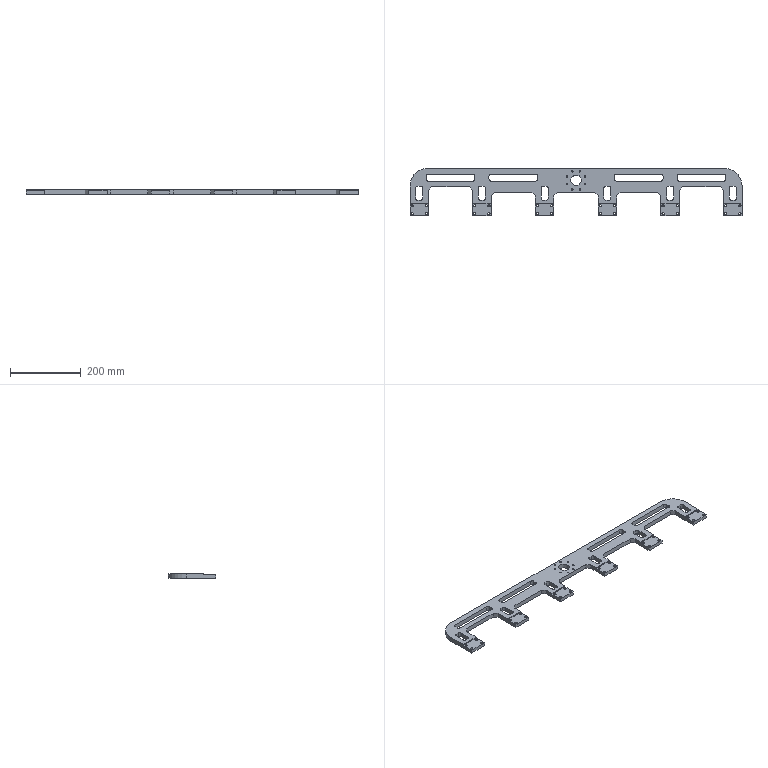NC program | NX | posted with a generic post | part box 941 x 134 x 13 mm
Lines 73 to 1151 of 4152:
(ZLEVEL_PROFILE_COPY_3_COPY_1 , TOOL : D10)
N132 T10 M6
N134 G54
N136 G17 G0 G90 X50.491 Y75.6 S9500 M3
N138 G43 Z30. H10
N140 Z4.036
N142 G94 G1 Z-0.964 F1000.
N144 X52.223 Y72.6
N146 G3 X53.089 Y72.1 R1.
N148 G1 X420.5 F3500.
N150 G2 X475.6 Y17. R55.1
N152 G1 Y-67.
N154 G2 X470.5 Y-72.1 R5.1
N156 G1 X418.5
N158 G2 X413.4 Y-67. R5.1
N160 G1 Y2.888
N162 X406.387 Y9.9
N164 X304.813
N166 X297.8 Y2.888
N168 Y-67.
N170 G2 X292.7 Y-72.1 R5.1
N172 G1 X240.7
N174 G2 X235.6 Y-67. R5.1
N176 G1 Y-13.067
N178 X228.588 Y-6.055
N180 X127.013
N182 X120. Y-13.068
N184 Y-67.
N186 G2 X114.9 Y-72.1 R5.1
N188 G1 X62.9
N190 G2 X57.8 Y-67. R5.1
N192 G1 Y-13.067
N194 X53.089 Y-8.357
N196 G3 X52.123 Y-8.098 R1.
N198 G1 X46.687 Y-9.555
N200 Z4.036
N202 G0 Z30.
N204 Z3.071
N206 G1 Z-1.929 F1000.
N208 X52.123 Y-8.098
N210 G2 X53.089 Y-8.357 R1.
N212 G1 X57.8 Y-13.067 F3500.
N214 Y-67.
N216 G3 X62.9 Y-72.1 R5.1
N218 G1 X114.9
N220 G3 X120. Y-67. R5.1
N222 G1 Y-13.068
N224 X127.013 Y-6.055
N226 X228.588
N228 X235.6 Y-13.067
N230 Y-67.
N232 G3 X240.7 Y-72.1 R5.1
N234 G1 X292.7
N236 G3 X297.8 Y-67. R5.1
N238 G1 Y2.888
N240 X304.813 Y9.9
N242 X406.387
N244 X413.4 Y2.888
N246 Y-67.
N248 G3 X418.5 Y-72.1 R5.1
N250 G1 X470.5
N252 G3 X475.6 Y-67. R5.1
N254 G1 Y17.
N256 G3 X420.5 Y72.1 R55.1
N258 G1 X53.089
N260 G2 X52.223 Y72.6 R1.
N262 G1 X50.491 Y75.6
N264 Z3.071
N266 G0 Z30.
N268 Z2.107
N270 G1 Z-2.893 F1000.
N272 X52.223 Y72.6
N274 G3 X53.089 Y72.1 R1.
N276 G1 X420.5 F3500.
N278 G2 X475.6 Y17. R55.1
N280 G1 Y-67.
N282 G2 X470.5 Y-72.1 R5.1
N284 G1 X418.5
N286 G2 X413.4 Y-67. R5.1
N288 G1 Y2.888
N290 X406.387 Y9.9
N292 X304.813
N294 X297.8 Y2.888
N296 Y-67.
N298 G2 X292.7 Y-72.1 R5.1
N300 G1 X240.7
N302 G2 X235.6 Y-67. R5.1
N304 G1 Y-13.067
N306 X228.588 Y-6.055
N308 X127.013
N310 X120. Y-13.068
N312 Y-67.
N314 G2 X114.9 Y-72.1 R5.1
N316 G1 X62.9
N318 G2 X57.8 Y-67. R5.1
N320 G1 Y-13.067
N322 X53.089 Y-8.357
N324 G3 X52.123 Y-8.098 R1.
N326 G1 X46.687 Y-9.555
N328 Z2.107
N330 G0 Z30.
N332 Z1.143
N334 G1 Z-3.857 F1000.
N336 X52.123 Y-8.098
N338 G2 X53.089 Y-8.357 R1.
N340 G1 X57.8 Y-13.067 F3500.
N342 Y-67.
N344 G3 X62.9 Y-72.1 R5.1
N346 G1 X114.9
N348 G3 X120. Y-67. R5.1
N350 G1 Y-13.068
N352 X127.013 Y-6.055
N354 X228.588
N356 X235.6 Y-13.067
N358 Y-67.
N360 G3 X240.7 Y-72.1 R5.1
N362 G1 X292.7
N364 G3 X297.8 Y-67. R5.1
N366 G1 Y2.888
N368 X304.813 Y9.9
N370 X406.387
N372 X413.4 Y2.888
N374 Y-67.
N376 G3 X418.5 Y-72.1 R5.1
N378 G1 X470.5
N380 G3 X475.6 Y-67. R5.1
N382 G1 Y17.
N384 G3 X420.5 Y72.1 R55.1
N386 G1 X53.089
N388 G2 X52.223 Y72.6 R1.
N390 G1 X50.491 Y75.6
N392 Z1.143
N394 G0 Z30.
N396 Z0.179
N398 G1 Z-4.821 F1000.
N400 X52.223 Y72.6
N402 G3 X53.089 Y72.1 R1.
N404 G1 X420.5 F3500.
N406 G2 X475.6 Y17. R55.1
N408 G1 Y-67.
N410 G2 X470.5 Y-72.1 R5.1
N412 G1 X418.5
N414 G2 X413.4 Y-67. R5.1
N416 G1 Y2.888
N418 X406.387 Y9.9
N420 X304.813
N422 X297.8 Y2.888
N424 Y-67.
N426 G2 X292.7 Y-72.1 R5.1
N428 G1 X240.7
N430 G2 X235.6 Y-67. R5.1
N432 G1 Y-13.067
N434 X228.588 Y-6.055
N436 X127.013
N438 X120. Y-13.068
N440 Y-67.
N442 G2 X114.9 Y-72.1 R5.1
N444 G1 X62.9
N446 G2 X57.8 Y-67. R5.1
N448 G1 Y-13.067
N450 X53.089 Y-8.357
N452 G3 X52.123 Y-8.098 R1.
N454 G1 X46.687 Y-9.555
N456 Z0.179
N458 G0 Z30.
N460 Z-0.786
N462 G1 Z-5.786 F1000.
N464 X52.123 Y-8.098
N466 G2 X53.089 Y-8.357 R1.
N468 G1 X57.8 Y-13.067 F3500.
N470 Y-67.
N472 G3 X62.9 Y-72.1 R5.1
N474 G1 X114.9
N476 G3 X120. Y-67. R5.1
N478 G1 Y-13.068
N480 X127.013 Y-6.055
N482 X228.588
N484 X235.6 Y-13.067
N486 Y-67.
N488 G3 X240.7 Y-72.1 R5.1
N490 G1 X292.7
N492 G3 X297.8 Y-67. R5.1
N494 G1 Y2.888
N496 X304.813 Y9.9
N498 X406.387
N500 X413.4 Y2.888
N502 Y-67.
N504 G3 X418.5 Y-72.1 R5.1
N506 G1 X470.5
N508 G3 X475.6 Y-67. R5.1
N510 G1 Y17.
N512 G3 X420.5 Y72.1 R55.1
N514 G1 X53.089
N516 G2 X52.223 Y72.6 R1.
N518 G1 X50.491 Y75.6
N520 Z-0.786
N522 G0 Z30.
N524 Z-1.75
N526 G1 Z-6.75 F1000.
N528 X52.223 Y72.6
N530 G3 X53.089 Y72.1 R1.
N532 G1 X420.5 F3500.
N534 G2 X475.6 Y17. R55.1
N536 G1 Y-67.
N538 G2 X470.5 Y-72.1 R5.1
N540 G1 X418.5
N542 G2 X413.4 Y-67. R5.1
N544 G1 Y2.888
N546 X406.387 Y9.9
N548 X304.813
N550 X297.8 Y2.888
N552 Y-67.
N554 G2 X292.7 Y-72.1 R5.1
N556 G1 X240.7
N558 G2 X235.6 Y-67. R5.1
N560 G1 Y-13.067
N562 X228.588 Y-6.055
N564 X127.013
N566 X120. Y-13.068
N568 Y-67.
N570 G2 X114.9 Y-72.1 R5.1
N572 G1 X62.9
N574 G2 X57.8 Y-67. R5.1
N576 G1 Y-13.067
N578 X53.089 Y-8.357
N580 G3 X52.123 Y-8.098 R1.
N582 G1 X46.687 Y-9.555
N584 Z-1.75
N586 G0 Z30.
N588 Z-2.714
N590 G1 Z-7.714 F1000.
N592 X52.123 Y-8.098
N594 G2 X53.089 Y-8.357 R1.
N596 G1 X57.8 Y-13.067 F3500.
N598 Y-67.
N600 G3 X62.9 Y-72.1 R5.1
N602 G1 X114.9
N604 G3 X120. Y-67. R5.1
N606 G1 Y-13.068
N608 X127.013 Y-6.055
N610 X228.588
N612 X235.6 Y-13.067
N614 Y-67.
N616 G3 X240.7 Y-72.1 R5.1
N618 G1 X292.7
N620 G3 X297.8 Y-67. R5.1
N622 G1 Y2.888
N624 X304.813 Y9.9
N626 X406.387
N628 X413.4 Y2.888
N630 Y-67.
N632 G3 X418.5 Y-72.1 R5.1
N634 G1 X470.5
N636 G3 X475.6 Y-67. R5.1
N638 G1 Y17.
N640 G3 X420.5 Y72.1 R55.1
N642 G1 X53.089
N644 G2 X52.223 Y72.6 R1.
N646 G1 X50.491 Y75.6
N648 Z-2.714
N650 G0 Z30.
N652 Z-3.679
N654 G1 Z-8.679 F1000.
N656 X52.223 Y72.6
N658 G3 X53.089 Y72.1 R1.
N660 G1 X420.5 F3500.
N662 G2 X475.6 Y17. R55.1
N664 G1 Y-67.
N666 G2 X470.5 Y-72.1 R5.1
N668 G1 X418.5
N670 G2 X413.4 Y-67. R5.1
N672 G1 Y2.888
N674 X406.388 Y9.9
N676 X304.812
N678 X297.8 Y2.888
N680 Y-67.
N682 G2 X292.7 Y-72.1 R5.1
N684 G1 X240.7
N686 G2 X235.6 Y-67. R5.1
N688 G1 Y-13.067
N690 X228.588 Y-6.055
N692 X127.012
N694 X120. Y-13.067
N696 Y-67.
N698 G2 X114.9 Y-72.1 R5.1
N700 G1 X62.9
N702 G2 X57.8 Y-67. R5.1
N704 G1 Y-13.067
N706 X53.089 Y-8.357
N708 G3 X52.123 Y-8.098 R1.
N710 G1 X46.686 Y-9.555
N712 Z-3.679
N714 G0 Z30.
N716 Z-4.643
N718 G1 Z-9.643 F1000.
N720 X52.123 Y-8.098
N722 G2 X53.089 Y-8.357 R1.
N724 G1 X57.8 Y-13.067 F3500.
N726 Y-67.
N728 G3 X62.9 Y-72.1 R5.1
N730 G1 X114.9
N732 G3 X120. Y-67. R5.1
N734 G1 Y-13.067
N736 X127.012 Y-6.055
N738 X228.588
N740 X235.6 Y-13.067
N742 Y-67.
N744 G3 X240.7 Y-72.1 R5.1
N746 G1 X292.7
N748 G3 X297.8 Y-67. R5.1
N750 G1 Y2.888
N752 X304.812 Y9.9
N754 X406.388
N756 X413.4 Y2.888
N758 Y-67.
N760 G3 X418.5 Y-72.1 R5.1
N762 G1 X470.5
N764 G3 X475.6 Y-67. R5.1
N766 G1 Y17.
N768 G3 X420.5 Y72.1 R55.1
N770 G1 X53.089
N772 G2 X52.223 Y72.6 R1.
N774 G1 X50.491 Y75.6
N776 Z-4.643
N778 G0 Z30.
N780 Z-5.607
N782 G1 Z-10.607 F1000.
N784 X52.223 Y72.6
N786 G3 X53.089 Y72.1 R1.
N788 G1 X420.5 F3500.
N790 G2 X475.6 Y17. R55.1
N792 G1 Y-67.
N794 G2 X470.5 Y-72.1 R5.1
N796 G1 X418.5
N798 G2 X413.4 Y-67. R5.1
N800 G1 Y2.888
N802 X406.388 Y9.9
N804 X304.812
N806 X297.8 Y2.888
N808 Y-67.
N810 G2 X292.7 Y-72.1 R5.1
N812 G1 X240.7
N814 G2 X235.6 Y-67. R5.1
N816 G1 Y-13.067
N818 X228.588 Y-6.055
N820 X127.012
N822 X120. Y-13.067
N824 Y-67.
N826 G2 X114.9 Y-72.1 R5.1
N828 G1 X62.9
N830 G2 X57.8 Y-67. R5.1
N832 G1 Y-13.067
N834 X53.089 Y-8.357
N836 G3 X52.123 Y-8.098 R1.
N838 G1 X46.686 Y-9.555
N840 Z-5.607
N842 G0 Z30.
N844 Z-6.571
N846 G1 Z-11.571 F1000.
N848 X52.123 Y-8.098
N850 G2 X53.089 Y-8.357 R1.
N852 G1 X57.8 Y-13.067 F3500.
N854 Y-67.
N856 G3 X62.9 Y-72.1 R5.1
N858 G1 X114.9
N860 G3 X120. Y-67. R5.1
N862 G1 Y-13.067
N864 X127.012 Y-6.055
N866 X228.588
N868 X235.6 Y-13.067
N870 Y-67.
N872 G3 X240.7 Y-72.1 R5.1
N874 G1 X292.7
N876 G3 X297.8 Y-67. R5.1
N878 G1 Y2.888
N880 X304.812 Y9.9
N882 X406.388
N884 X413.4 Y2.888
N886 Y-67.
N888 G3 X418.5 Y-72.1 R5.1
N890 G1 X470.5
N892 G3 X475.6 Y-67. R5.1
N894 G1 Y17.
N896 G3 X420.5 Y72.1 R55.1
N898 G1 X53.089
N900 G2 X52.223 Y72.6 R1.
N902 G1 X50.491 Y75.6
N904 Z-6.571
N906 G0 Z30.
N908 Z-7.536
N910 G1 Z-12.536 F1000.
N912 X52.223 Y72.6
N914 G3 X53.089 Y72.1 R1.
N916 G1 X420.5 F3500.
N918 G2 X475.6 Y17. R55.1
N920 G1 Y-67.
N922 G2 X470.5 Y-72.1 R5.1
N924 G1 X418.5
N926 G2 X413.4 Y-67. R5.1
N928 G1 Y2.888
N930 X406.388 Y9.9
N932 X304.812
N934 X297.8 Y2.888
N936 Y-67.
N938 G2 X292.7 Y-72.1 R5.1
N940 G1 X240.7
N942 G2 X235.6 Y-67. R5.1
N944 G1 Y-13.067
N946 X228.588 Y-6.055
N948 X127.012
N950 X120. Y-13.067
N952 Y-67.
N954 G2 X114.9 Y-72.1 R5.1
N956 G1 X62.9
N958 G2 X57.8 Y-67. R5.1
N960 G1 Y-13.067
N962 X53.089 Y-8.357
N964 G3 X52.123 Y-8.098 R1.
N966 G1 X46.686 Y-9.555
N968 Z-7.536
N970 G0 Z30.
N972 Z-8.5
N974 G1 Z-13.5 F1000.
N976 X52.123 Y-8.098
N978 G2 X53.089 Y-8.357 R1.
N980 G1 X57.8 Y-13.067 F3500.
N982 Y-67.
N984 G3 X62.9 Y-72.1 R5.1
N986 G1 X114.9
N988 G3 X120. Y-67. R5.1
N990 G1 Y-13.067
N992 X127.012 Y-6.055
N994 X228.588
N996 X235.6 Y-13.067
N998 Y-67.
N1000 G3 X240.7 Y-72.1 R5.1
N1002 G1 X292.7
N1004 G3 X297.8 Y-67. R5.1
N1006 G1 Y2.888
N1008 X304.812 Y9.9
N1010 X406.388
N1012 X413.4 Y2.888
N1014 Y-67.
N1016 G3 X418.5 Y-72.1 R5.1
N1018 G1 X470.5
N1020 G3 X475.6 Y-67. R5.1
N1022 G1 Y17.
N1024 G3 X420.5 Y72.1 R55.1
N1026 G1 X53.089
N1028 G2 X52.223 Y72.6 R1.
N1030 G1 X50.491 Y75.6
N1032 Z-8.5
N1034 G0 Z30.
(ZLEVEL_PROFILE_COPY_3_COPY_COPY , TOOL : D10)
N1036 Y75.5
N1038 Z-8.5
N1040 G1 Z-13.5 F1000.
N1042 X52.223 Y72.5
N1044 G3 X53.089 Y72. R1.
N1046 G1 X420.5 F1200.
N1048 G2 X475.5 Y17. R55.
N1050 G1 Y-67.
N1052 G2 X470.5 Y-72. R5.
N1054 G1 X418.5
N1056 G2 X413.5 Y-67. R5.
N1058 G1 Y2.929
N1060 X406.429 Y10.
N1062 X304.771
N1064 X297.7 Y2.929
N1066 Y-67.
N1068 G2 X292.7 Y-72. R5.
N1070 G1 X240.7
N1072 G2 X235.7 Y-67. R5.
N1074 G1 Y-13.026
N1076 X228.629 Y-5.955
N1078 X126.971
N1080 X119.9 Y-13.026
N1082 Y-67.
N1084 G2 X114.9 Y-72. R5.
N1086 G1 X62.9
N1088 G2 X57.9 Y-67. R5.
N1090 G1 Y-13.026
N1092 X53.089 Y-8.215
N1094 G3 X52.123 Y-7.957 R1.
N1096 G1 X46.531 Y-9.455
N1098 Z-8.5
N1100 G0 Z30.
(ZLEVEL_PROFILE_COPY_2_COPY_COPY_1 , TOOL : D10)
N1102 X402.621 Y45.9
N1104 Z1.5
N1106 G1 X355.6 Z-0.964 F1000.
N1108 X292.7 F3500.
N1110 G3 X291.8 Y45. R0.9
N1112 G1 Y37.
N1114 G3 X292.7 Y36.1 R0.9
N1116 G1 X418.5
N1118 G3 X419.4 Y37. R0.9
N1120 G1 Y45.
N1122 G3 X418.5 Y45.9 R0.9
N1124 G1 X355.6
N1126 X300.356 Z-1.929
N1128 X292.7
N1130 G3 X291.8 Y45. R0.9
N1132 G1 Y37.
N1134 G3 X292.7 Y36.1 R0.9
N1136 G1 X418.5
N1138 G3 X419.4 Y37. R0.9
N1140 G1 Y45.
N1142 G3 X418.5 Y45.9 R0.9
N1144 G1 X355.6
N1146 X300.356 Z-2.893
N1148 X292.7
N1150 G3 X291.8 Y45. R0.9
N1152 G1 Y37.
N1154 G3 X292.7 Y36.1 R0.9
N1156 G1 X418.5
N1158 G3 X419.4 Y37. R0.9
N1160 G1 Y45.
N1162 G3 X418.5 Y45.9 R0.9
N1164 G1 X355.6
N1166 X300.356 Z-3.857
N1168 X292.7
N1170 G3 X291.8 Y45. R0.9
N1172 G1 Y37.
N1174 G3 X292.7 Y36.1 R0.9
N1176 G1 X418.5
N1178 G3 X419.4 Y37. R0.9
N1180 G1 Y45.
N1182 G3 X418.5 Y45.9 R0.9
N1184 G1 X355.6
N1186 X300.356 Z-4.821
N1188 X292.7
N1190 G3 X291.8 Y45. R0.9
N1192 G1 Y37.
N1194 G3 X292.7 Y36.1 R0.9
N1196 G1 X418.5
N1198 G3 X419.4 Y37. R0.9
N1200 G1 Y45.
N1202 G3 X418.5 Y45.9 R0.9
N1204 G1 X355.6
N1206 X300.356 Z-5.786
N1208 X292.7
N1210 G3 X291.8 Y45. R0.9
N1212 G1 Y37.
N1214 G3 X292.7 Y36.1 R0.9
N1216 G1 X418.5
N1218 G3 X419.4 Y37. R0.9
N1220 G1 Y45.
N1222 G3 X418.5 Y45.9 R0.9
N1224 G1 X355.6
N1226 X300.356 Z-6.75
N1228 X292.7
N1230 G3 X291.8 Y45. R0.9
N1232 G1 Y37.
N1234 G3 X292.7 Y36.1 R0.9
N1236 G1 X418.5
N1238 G3 X419.4 Y37. R0.9
N1240 G1 Y45.
N1242 G3 X418.5 Y45.9 R0.9
N1244 G1 X355.6
N1246 X300.356 Z-7.714
N1248 X292.7
N1250 G3 X291.8 Y45. R0.9
N1252 G1 Y37.
N1254 G3 X292.7 Y36.1 R0.9
N1256 G1 X418.5
N1258 G3 X419.4 Y37. R0.9
N1260 G1 Y45.
N1262 G3 X418.5 Y45.9 R0.9
N1264 G1 X355.6
N1266 X300.356 Z-8.679
N1268 X292.7
N1270 G3 X291.8 Y45. R0.9
N1272 G1 Y37.
N1274 G3 X292.7 Y36.1 R0.9
N1276 G1 X418.5
N1278 G3 X419.4 Y37. R0.9
N1280 G1 Y45.
N1282 G3 X418.5 Y45.9 R0.9
N1284 G1 X355.6
N1286 X300.356 Z-9.643
N1288 X292.7
N1290 G3 X291.8 Y45. R0.9
N1292 G1 Y37.
N1294 G3 X292.7 Y36.1 R0.9
N1296 G1 X418.5
N1298 G3 X419.4 Y37. R0.9
N1300 G1 Y45.
N1302 G3 X418.5 Y45.9 R0.9
N1304 G1 X355.6
N1306 X300.356 Z-10.607
N1308 X292.7
N1310 G3 X291.8 Y45. R0.9
N1312 G1 Y37.
N1314 G3 X292.7 Y36.1 R0.9
N1316 G1 X418.5
N1318 G3 X419.4 Y37. R0.9
N1320 G1 Y45.
N1322 G3 X418.5 Y45.9 R0.9
N1324 G1 X355.6
N1326 X300.356 Z-11.571
N1328 X292.7
N1330 G3 X291.8 Y45. R0.9
N1332 G1 Y37.
N1334 G3 X292.7 Y36.1 R0.9
N1336 G1 X418.5
N1338 G3 X419.4 Y37. R0.9
N1340 G1 Y45.
N1342 G3 X418.5 Y45.9 R0.9
N1344 G1 X355.6
N1346 X300.356 Z-12.536
N1348 X292.7
N1350 G3 X291.8 Y45. R0.9
N1352 G1 Y37.
N1354 G3 X292.7 Y36.1 R0.9
N1356 G1 X418.5
N1358 G3 X419.4 Y37. R0.9
N1360 G1 Y45.
N1362 G3 X418.5 Y45.9 R0.9
N1364 G1 X355.6
N1366 X300.356 Z-13.5
N1368 X292.7
N1370 G3 X291.8 Y45. R0.9
N1372 G1 Y37.
N1374 G3 X292.7 Y36.1 R0.9
N1376 G1 X418.5
N1378 G3 X419.4 Y37. R0.9
N1380 G1 Y45.
N1382 G3 X418.5 Y45.9 R0.9
N1384 G1 X300.356
N1386 Z-12.
N1388 G0 Z30.
N1390 X224.821
N1392 Z1.5
N1394 G1 X177.8 Z-0.964 F1000.
N1396 X114.9 F3500.
N1398 G3 X114. Y45. R0.9
N1400 G1 Y37.
N1402 G3 X114.9 Y36.1 R0.9
N1404 G1 X240.7
N1406 G3 X241.6 Y37. R0.9
N1408 G1 Y45.
N1410 G3 X240.7 Y45.9 R0.9
N1412 G1 X177.8
N1414 X122.556 Z-1.929
N1416 X114.9
N1418 G3 X114. Y45. R0.9
N1420 G1 Y37.
N1422 G3 X114.9 Y36.1 R0.9
N1424 G1 X240.7
N1426 G3 X241.6 Y37. R0.9
N1428 G1 Y45.
N1430 G3 X240.7 Y45.9 R0.9
N1432 G1 X177.8
N1434 X122.556 Z-2.893
N1436 X114.9
N1438 G3 X114. Y45. R0.9
N1440 G1 Y37.
N1442 G3 X114.9 Y36.1 R0.9
N1444 G1 X240.7
N1446 G3 X241.6 Y37. R0.9
N1448 G1 Y45.
N1450 G3 X240.7 Y45.9 R0.9
N1452 G1 X177.8
N1454 X122.556 Z-3.857
N1456 X114.9
N1458 G3 X114. Y45. R0.9
N1460 G1 Y37.
N1462 G3 X114.9 Y36.1 R0.9
N1464 G1 X240.7
N1466 G3 X241.6 Y37. R0.9
N1468 G1 Y45.
N1470 G3 X240.7 Y45.9 R0.9
N1472 G1 X177.8
N1474 X122.556 Z-4.821
N1476 X114.9
N1478 G3 X114. Y45. R0.9
N1480 G1 Y37.
N1482 G3 X114.9 Y36.1 R0.9
N1484 G1 X240.7
N1486 G3 X241.6 Y37. R0.9
N1488 G1 Y45.
N1490 G3 X240.7 Y45.9 R0.9
N1492 G1 X177.8
N1494 X122.556 Z-5.786
N1496 X114.9
N1498 G3 X114. Y45. R0.9
N1500 G1 Y37.
N1502 G3 X114.9 Y36.1 R0.9
N1504 G1 X240.7
N1506 G3 X241.6 Y37. R0.9
N1508 G1 Y45.
N1510 G3 X240.7 Y45.9 R0.9
N1512 G1 X177.8
N1514 X122.556 Z-6.75
N1516 X114.9
N1518 G3 X114. Y45. R0.9
N1520 G1 Y37.
N1522 G3 X114.9 Y36.1 R0.9
N1524 G1 X240.7
N1526 G3 X241.6 Y37. R0.9
N1528 G1 Y45.
N1530 G3 X240.7 Y45.9 R0.9
N1532 G1 X177.8
N1534 X122.556 Z-7.714
N1536 X114.9
N1538 G3 X114. Y45. R0.9
N1540 G1 Y37.
N1542 G3 X114.9 Y36.1 R0.9
N1544 G1 X240.7
N1546 G3 X241.6 Y37. R0.9
N1548 G1 Y45.
N1550 G3 X240.7 Y45.9 R0.9
N1552 G1 X177.8
N1554 X122.556 Z-8.679
N1556 X114.9
N1558 G3 X114. Y45. R0.9
N1560 G1 Y37.
N1562 G3 X114.9 Y36.1 R0.9
N1564 G1 X240.7
N1566 G3 X241.6 Y37. R0.9
N1568 G1 Y45.
N1570 G3 X240.7 Y45.9 R0.9
N1572 G1 X177.8
N1574 X122.556 Z-9.643
N1576 X114.9
N1578 G3 X114. Y45. R0.9
N1580 G1 Y37.
N1582 G3 X114.9 Y36.1 R0.9
N1584 G1 X240.7
N1586 G3 X241.6 Y37. R0.9
N1588 G1 Y45.
N1590 G3 X240.7 Y45.9 R0.9
N1592 G1 X177.8
N1594 X122.556 Z-10.607
N1596 X114.9
N1598 G3 X114. Y45. R0.9
N1600 G1 Y37.
N1602 G3 X114.9 Y36.1 R0.9
N1604 G1 X240.7
N1606 G3 X241.6 Y37. R0.9
N1608 G1 Y45.
N1610 G3 X240.7 Y45.9 R0.9
N1612 G1 X177.8
N1614 X122.556 Z-11.571
N1616 X114.9
N1618 G3 X114. Y45. R0.9
N1620 G1 Y37.
N1622 G3 X114.9 Y36.1 R0.9
N1624 G1 X240.7
N1626 G3 X241.6 Y37. R0.9
N1628 G1 Y45.
N1630 G3 X240.7 Y45.9 R0.9
N1632 G1 X177.8
N1634 X122.556 Z-12.536
N1636 X114.9
N1638 G3 X114. Y45. R0.9
N1640 G1 Y37.
N1642 G3 X114.9 Y36.1 R0.9
N1644 G1 X240.7
N1646 G3 X241.6 Y37. R0.9
N1648 G1 Y45.
N1650 G3 X240.7 Y45.9 R0.9
N1652 G1 X177.8
N1654 X122.556 Z-13.5
N1656 X114.9
N1658 G3 X114. Y45. R0.9
N1660 G1 Y37.
N1662 G3 X114.9 Y36.1 R0.9
N1664 G1 X240.7
N1666 G3 X241.6 Y37. R0.9
N1668 G1 Y45.
N1670 G3 X240.7 Y45.9 R0.9
N1672 G1 X122.556
N1674 Z-12.
N1676 G0 Z30.
N1678 X439.6 Y4.774
N1680 Z1.5
N1682 G1 Y-17.535 Z0.331 F1000.
N1684 X439.687 Y-17.81 Z0.316
N1686 X439.857 Y-18.043 Z0.301
N1688 X440.09 Y-18.213 Z0.285
N1690 X440.365 Y-18.3 Z0.27
N1692 X448.635 Z-0.163
N1694 X448.91 Y-18.213 Z-0.178
N1696 X449.143 Y-18.043 Z-0.193
N1698 X449.313 Y-17.81 Z-0.208
N1700 X449.4 Y-17.535 Z-0.224
N1702 Y-3.4 Z-0.964
N1704 Y10.6 F3500.
N1706 G3 X448.5 Y11.5 R0.9
N1708 G1 X440.5
N1710 G3 X439.6 Y10.6 R0.9
N1712 G1 Y-17.4
N1714 G3 X440.5 Y-18.3 R0.9
N1716 G1 X448.5
N1718 G3 X449.4 Y-17.4 R0.9
N1720 G1 Y-3.4
N1722 Y10.411 Z-1.205
N1724 X449.389 Y10.65 Z-1.21
N1726 X449.376 Y10.768 Z-1.212
N1728 X449.371 Y10.796
N1730 X449.355 Y10.851 Z-1.213
N1732 X449.279 Y11.033 Z-1.217
N1734 X449.228 Y11.114 Z-1.218
N1736 X449.2 Y11.154 Z-1.219
N1738 X449.135 Y11.228 Z-1.221
N1740 X449.001 Y11.336 Z-1.224
N1742 X448.93 Y11.381 Z-1.225
N1744 X448.875 Y11.41 Z-1.227
N1746 X448.76 Y11.453 Z-1.229
N1748 X448.673 Y11.474 Z-1.23
N1750 X448.629 Y11.482 Z-1.231
N1752 X448.527 Y11.491 Z-1.233
N1754 X448.321 Y11.5 Z-1.236
N1756 X440.747 Z-1.369
N1758 X440.365 Y11.482 Z-1.375
N1760 X440.305 Y11.471 Z-1.376
N1762 X440.13 Y11.412 Z-1.38
N1764 X440.05 Y11.371 Z-1.381
N1766 X440.003 Y11.341 Z-1.382
N1768 X439.915 Y11.273 Z-1.384
N1770 X439.794 Y11.144 Z-1.387
N1772 X439.742 Y11.073 Z-1.389
N1774 X439.715 Y11.021 Z-1.39
N1776 X439.666 Y10.914 Z-1.392
N1778 X439.635 Y10.816 Z-1.394
N1780 X439.624 Y10.765 Z-1.395
N1782 X439.612 Y10.671 Z-1.396
N1784 X439.6 Y10.479 Z-1.4
N1786 Y-17.143 Z-1.882
N1788 X439.62 Y-17.587 Z-1.89
N1790 X439.665 Y-17.737 Z-1.892
N1792 X439.697 Y-17.806 Z-1.894
N1794 X439.731 Y-17.867 Z-1.895
N1796 X439.821 Y-17.978 Z-1.897
N1798 X439.956 Y-18.108 Z-1.901
N1800 X440.032 Y-18.16 Z-1.902
N1802 X440.079 Y-18.186 Z-1.903
N1804 X440.177 Y-18.231 Z-1.905
N1806 X440.277 Y-18.264 Z-1.907
N1808 X440.329 Y-18.275 Z-1.908
N1810 X440.422 Y-18.288 Z-1.91
N1812 X440.612 Y-18.298 Z-1.913
N1814 X440.834 Y-18.3 Z-1.917
N1816 X441.503 Z-1.929
N1818 X448.5
N1820 G3 X449.4 Y-17.4 R0.9
N1822 G1 Y-3.4
N1824 Y10.411 Z-2.17
N1826 X449.389 Y10.65 Z-2.174
N1828 X449.376 Y10.768 Z-2.176
N1830 X449.371 Y10.796
N1832 X449.355 Y10.851 Z-2.177
N1834 X449.279 Y11.033 Z-2.181
N1836 X449.228 Y11.114 Z-2.183
N1838 X449.2 Y11.154
N1840 X449.135 Y11.228 Z-2.185
N1842 X449.001 Y11.336 Z-2.188
N1844 X448.93 Y11.381 Z-2.19
N1846 X448.875 Y11.41 Z-2.191
N1848 X448.76 Y11.453 Z-2.193
N1850 X448.673 Y11.474 Z-2.195
N1852 X448.629 Y11.482
N1854 X448.527 Y11.491 Z-2.197
N1856 X448.321 Y11.5 Z-2.201
N1858 X440.747 Z-2.333
N1860 X440.365 Y11.482 Z-2.34
N1862 X440.305 Y11.471 Z-2.341
N1864 X440.13 Y11.412 Z-2.344
N1866 X440.05 Y11.371 Z-2.346
N1868 X440.003 Y11.341 Z-2.347
N1870 X439.915 Y11.273 Z-2.349
N1872 X439.794 Y11.144 Z-2.352
N1874 X439.742 Y11.073 Z-2.353
N1876 X439.715 Y11.021 Z-2.354
N1878 X439.666 Y10.914 Z-2.356
N1880 X439.635 Y10.816 Z-2.358
N1882 X439.624 Y10.765 Z-2.359
N1884 X439.61 Y10.671 Z-2.361
N1886 X439.6 Y10.479 Z-2.364
N1888 Y-17.143 Z-2.846
N1890 X439.62 Y-17.587 Z-2.854
N1892 X439.665 Y-17.737 Z-2.857
N1894 X439.697 Y-17.806 Z-2.858
N1896 X439.731 Y-17.867 Z-2.859
N1898 X439.821 Y-17.978 Z-2.862
N1900 X439.956 Y-18.108 Z-2.865
N1902 X440.032 Y-18.16 Z-2.867
N1904 X440.079 Y-18.186 Z-2.868
N1906 X440.177 Y-18.231 Z-2.87
N1908 X440.277 Y-18.264 Z-2.871
N1910 X440.329 Y-18.275 Z-2.872
N1912 X440.422 Y-18.288 Z-2.874
N1914 X440.612 Y-18.298 Z-2.877
N1916 X440.834 Y-18.3 Z-2.881
N1918 X441.503 Z-2.893
N1920 X448.5
N1922 G3 X449.4 Y-17.4 R0.9
N1924 G1 Y-3.4
N1926 Y10.411 Z-3.134
N1928 X449.389 Y10.65 Z-3.138
N1930 X449.376 Y10.768 Z-3.14
N1932 X449.371 Y10.796 Z-3.141
N1934 X449.355 Y10.851 Z-3.142
N1936 X449.279 Y11.033 Z-3.145
N1938 X449.228 Y11.114 Z-3.147
N1940 X449.2 Y11.154 Z-3.148
N1942 X449.135 Y11.228 Z-3.149
N1944 X449.001 Y11.336 Z-3.152
N1946 X448.93 Y11.381 Z-3.154
N1948 X448.875 Y11.41 Z-3.155
N1950 X448.76 Y11.453 Z-3.157
N1952 X448.673 Y11.474 Z-3.159
N1954 X448.629 Y11.482 Z-3.16
N1956 X448.527 Y11.491 Z-3.161
N1958 X448.321 Y11.5 Z-3.165
N1960 X440.747 Z-3.297
N1962 X440.365 Y11.482 Z-3.304
N1964 X440.305 Y11.471 Z-3.305
N1966 X440.13 Y11.412 Z-3.308
N1968 X440.05 Y11.371 Z-3.31
N1970 X440.003 Y11.341 Z-3.311
N1972 X439.915 Y11.273 Z-3.313
N1974 X439.794 Y11.144 Z-3.316
N1976 X439.742 Y11.073 Z-3.317
N1978 X439.715 Y11.021 Z-3.318
N1980 X439.666 Y10.914 Z-3.321
N1982 X439.635 Y10.816 Z-3.322
N1984 X439.624 Y10.765 Z-3.323
N1986 X439.61 Y10.671 Z-3.325
N1988 X439.6 Y10.479 Z-3.328
N1990 Y-17.143 Z-3.81
N1992 X439.62 Y-17.587 Z-3.818
N1994 X439.665 Y-17.737 Z-3.821
N1996 X439.697 Y-17.806 Z-3.822
N1998 X439.731 Y-17.867 Z-3.824
N2000 X439.821 Y-17.978 Z-3.826
N2002 X439.956 Y-18.108 Z-3.829
N2004 X440.032 Y-18.16 Z-3.831
N2006 X440.079 Y-18.186 Z-3.832
N2008 X440.177 Y-18.231 Z-3.834
N2010 X440.277 Y-18.264 Z-3.836
N2012 X440.329 Y-18.275 Z-3.837
N2014 X440.422 Y-18.288 Z-3.838
N2016 X440.612 Y-18.298 Z-3.842
N2018 X440.834 Y-18.3 Z-3.845
N2020 X441.503 Z-3.857
N2022 X448.5
N2024 G3 X449.4 Y-17.4 R0.9
N2026 G1 Y-3.4
N2028 Y10.411 Z-4.098
N2030 X449.389 Y10.65 Z-4.102
N2032 X449.376 Y10.768 Z-4.104
N2034 X449.371 Y10.796 Z-4.105
N2036 X449.355 Y10.851 Z-4.106
N2038 X449.279 Y11.033 Z-4.109
N2040 X449.228 Y11.114 Z-4.111
N2042 X449.2 Y11.154 Z-4.112
N2044 X449.135 Y11.228 Z-4.114
N2046 X449.001 Y11.336 Z-4.117
N2048 X448.93 Y11.381 Z-4.118
N2050 X448.876 Y11.41 Z-4.119
N2052 X448.76 Y11.453 Z-4.122
N2054 X448.673 Y11.474 Z-4.123
N2056 X448.629 Y11.482 Z-4.124
N2058 X448.527 Y11.491 Z-4.126
N2060 X448.321 Y11.5 Z-4.129
N2062 X440.747 Z-4.262
N2064 X440.365 Y11.482 Z-4.268
N2066 X440.305 Y11.471 Z-4.269
N2068 X440.13 Y11.412 Z-4.272
N2070 X440.05 Y11.371 Z-4.274
N2072 X440.003 Y11.341 Z-4.275
N2074 X439.915 Y11.273 Z-4.277
N2076 X439.794 Y11.144 Z-4.28
N2078 X439.742 Y11.073 Z-4.282
N2080 X439.715 Y11.021 Z-4.283
N2082 X439.666 Y10.914 Z-4.285
N2084 X439.635 Y10.816 Z-4.287
N2086 X439.624 Y10.765 Z-4.288
N2088 X439.61 Y10.671 Z-4.289
N2090 X439.6 Y10.479 Z-4.293
N2092 Y-17.143 Z-4.775
N2094 X439.62 Y-17.587 Z-4.783
N2096 X439.665 Y-17.737 Z-4.785
N2098 X439.697 Y-17.806 Z-4.787
N2100 X439.731 Y-17.867 Z-4.788
N2102 X439.821 Y-17.978 Z-4.79
N2104 X439.957 Y-18.108 Z-4.794
N2106 X440.032 Y-18.16 Z-4.795
N2108 X440.079 Y-18.186 Z-4.796
N2110 X440.177 Y-18.231 Z-4.798
N2112 X440.277 Y-18.264 Z-4.8
N2114 X440.329 Y-18.275 Z-4.801
N2116 X440.422 Y-18.288 Z-4.803
N2118 X440.612 Y-18.298 Z-4.806
N2120 X440.834 Y-18.3 Z-4.81
N2122 X441.503 Z-4.821
N2124 X448.5
N2126 G3 X449.4 Y-17.4 R0.9
N2128 G1 Y-3.4
N2130 Y10.411 Z-5.063
N2132 X449.389 Y10.65 Z-5.067
N2134 X449.376 Y10.768 Z-5.069
N2136 X449.371 Y10.796
N2138 X449.355 Y10.851 Z-5.07
N2140 X449.279 Y11.033 Z-5.074
N2142 X449.228 Y11.114 Z-5.075
N2144 X449.2 Y11.154 Z-5.076
N2146 X449.135 Y11.228 Z-5.078
N2148 X449.001 Y11.336 Z-5.081
N2150 X448.93 Y11.381 Z-5.083
N2152 X448.876 Y11.41 Z-5.084
N2154 X448.76 Y11.453 Z-5.086
N2156 X448.673 Y11.474 Z-5.087
N2158 X448.629 Y11.482 Z-5.088
N2160 X448.527 Y11.491 Z-5.09
N2162 X448.321 Y11.5 Z-5.094
N2164 X440.747 Z-5.226
N2166 X440.365 Y11.482 Z-5.232
N2168 X440.305 Y11.471 Z-5.234
N2170 X440.13 Y11.412 Z-5.237
N2172 X440.05 Y11.371 Z-5.238
N2174 X440.003 Y11.341 Z-5.239
N2176 X439.915 Y11.273 Z-5.241
N2178 X439.792 Y11.144 Z-5.244
N2180 X439.742 Y11.073 Z-5.246
N2182 X439.715 Y11.021 Z-5.247
N2184 X439.666 Y10.914 Z-5.249
N2186 X439.635 Y10.816 Z-5.251
N2188 X439.624 Y10.765 Z-5.252
N2190 X439.61 Y10.671 Z-5.254
N2192 X439.6 Y10.479 Z-5.257
N2194 Y-17.143 Z-5.739
N2196 X439.62 Y-17.587 Z-5.747
N2198 X439.665 Y-17.737 Z-5.75
N2200 X439.697 Y-17.806 Z-5.751
N2202 X439.731 Y-17.867 Z-5.752
N2204 X439.821 Y-17.978 Z-5.755
N2206 X439.957 Y-18.108 Z-5.758
N2208 X440.032 Y-18.16 Z-5.76
N2210 X440.079 Y-18.186
N2212 X440.177 Y-18.231 Z-5.762
N2214 X440.277 Y-18.264 Z-5.764
N2216 X440.329 Y-18.275 Z-5.765
N2218 X440.422 Y-18.288 Z-5.767
N2220 X440.612 Y-18.298 Z-5.77
N2222 X440.834 Y-18.3 Z-5.774
N2224 X441.503 Z-5.786
N2226 X448.5
N2228 G3 X449.4 Y-17.4 R0.9
N2230 G1 Y-3.4
N2232 Y10.411 Z-6.027
N2234 X449.389 Y10.65 Z-6.031
N2236 X449.376 Y10.768 Z-6.033
N2238 X449.371 Y10.796 Z-6.034
N2240 X449.355 Y10.851 Z-6.035
N2242 X449.279 Y11.032 Z-6.038
N2244 X449.228 Y11.114 Z-6.04
N2246 X449.2 Y11.154 Z-6.041
N2248 X449.135 Y11.228 Z-6.042
N2250 X449.002 Y11.336 Z-6.045
N2252 X448.93 Y11.381 Z-6.047
N2254 X448.876 Y11.41 Z-6.048
N2256 X448.76 Y11.453 Z-6.05
N2258 X448.673 Y11.474 Z-6.052
N2260 X448.629 Y11.482
N2262 X448.527 Y11.491 Z-6.054
N2264 X448.321 Y11.5 Z-6.058
N2266 X440.747 Z-6.19
N2268 X440.365 Y11.482 Z-6.197
N2270 X440.305 Y11.471 Z-6.198